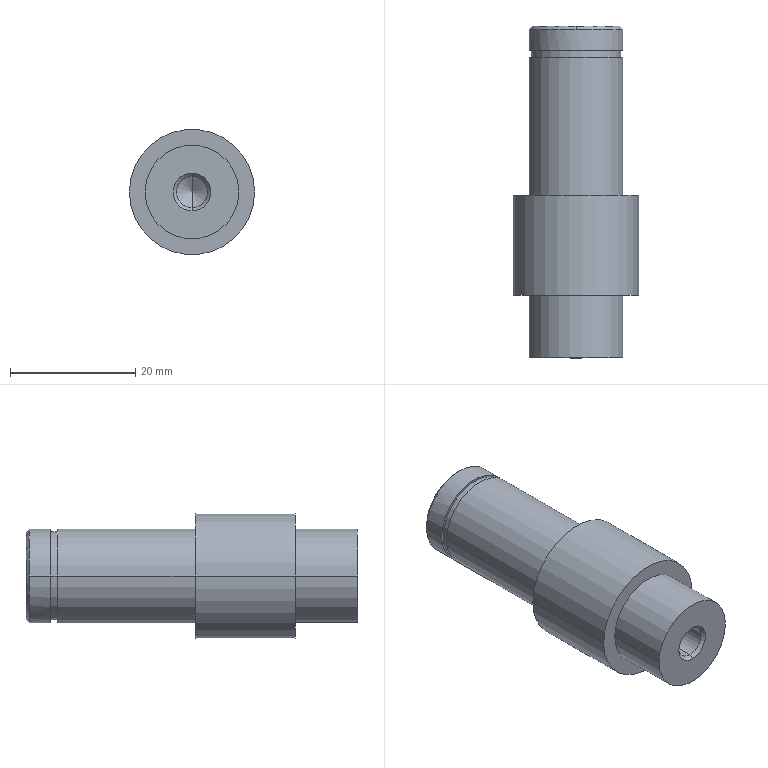Part | STEP file | 1 solid | 24 faces | box 20 x 53 x 20 mm | volume 11196 mm3 | cylinder 12 | cone 6 | plane 6 | commonest cylinder face diameters 15 x6 5 x2 14.3 x2 20 x2